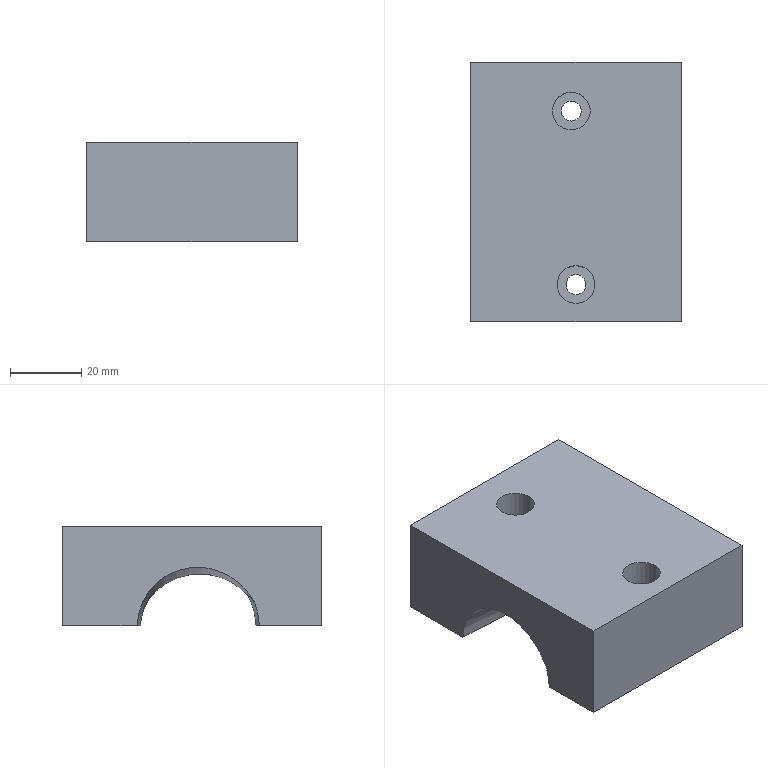NC program | NX | posted with a generic post | part box 59.014 x 72.744 x 27.972 mm
Lines 1691 to 2486 of 94199:
(FIXED_CONTOUR , TOOL : R2)
N3362 T11 M6
N3364 G54
N3366 G17 G0 G90 X17.129 Y-31.067 S9500 M3
N3368 G43 Z30. H11
N3370 Z5.2
N3372 G94 G1 Z0.147 F1000.
N3374 X17.141 Y-31.095
N3376 X17.133 Y-31.126
N3378 X17.108 Y-31.144
N3380 X17.106 Y-31.146 Z0.122 F3000.
N3382 X17.08 Y-31.172 Z-1.507
N3384 X17.056 Y-31.196 Z-2.477
N3386 X17.019 Y-31.233 Z-2.947
N3388 X16.997 Y-31.255 Z-3.192
N3390 X16.986 Y-31.266 Z-3.29
N3392 X16.964 Y-31.289 Z-3.454
N3394 X16.947 Y-31.29 Z-3.603
N3396 X16.9 Y-31.291 Z-3.934
N3398 X16.92 Y-31.272 Z-3.829
N3400 X16.962 Y-31.23 Z-3.571
N3402 X16.995 Y-31.197 Z-3.331
N3404 X17.012 Y-31.18 Z-3.182
N3406 X17.064 Y-31.127 Z-2.569
N3408 X17.076 Y-31.116 Z-2.344
N3410 X17.091 Y-31.101 Z-1.761
N3412 X17.122 Y-31.07 Z0.149
N3414 X17.127 Y-31.042 Z0.15
N3416 X17.095 Y-31.074 Z-1.856
N3418 X17.084 Y-31.085 Z-2.285
N3420 X17.067 Y-31.102 Z-2.61
N3422 X17.032 Y-31.137 Z-3.022
N3424 X17.018 Y-31.151 Z-3.175
N3426 X16.998 Y-31.171 Z-3.347
N3428 X16.969 Y-31.199 Z-3.555
N3430 X16.92 Y-31.249 Z-3.858
N3432 X16.877 Y-31.292 Z-4.088
N3434 X16.855 Y-31.293 Z-4.24
N3436 X16.92 Y-31.228 Z-3.886
N3438 X16.977 Y-31.171 Z-3.54
N3440 X17.001 Y-31.146 Z-3.361
N3442 X17.028 Y-31.119 Z-3.116
N3444 X17.043 Y-31.105 Z-2.966
N3446 X17.069 Y-31.078 Z-2.65
N3448 X17.091 Y-31.056 Z-2.23
N3450 X17.098 Y-31.049 Z-1.945
N3452 X17.132 Y-31.016 Z0.15
N3454 X17.137 Y-30.988 Z0.151
N3456 X17.102 Y-31.023 Z-2.038
N3458 X17.099 Y-31.026 Z-2.172
N3460 X17.072 Y-31.054 Z-2.691
N3462 X17.044 Y-31.082 Z-3.01
N3464 X17.019 Y-31.106 Z-3.244
N3466 X17.004 Y-31.121 Z-3.376
N3468 X16.984 Y-31.141 Z-3.524
N3470 X16.92 Y-31.206 Z-3.916
N3472 X16.851 Y-31.274 Z-4.289
N3474 X16.831 Y-31.294 Z-4.379
N3476 X16.805 Z-4.523
N3478 X16.86 Y-31.239 Z-4.276
N3480 X16.92 Y-31.179 Z-3.95
N3482 X16.993 Y-31.106 Z-3.505
N3484 X17.008 Y-31.091 Z-3.394
N3486 X17.019 Y-31.08 Z-3.295
N3488 X17.066 Y-31.033 Z-2.839
N3490 X17.074 Y-31.024 Z-2.739
N3492 X17.107 Y-30.991 Z-2.114
N3494 X17.143 Y-30.956 Z0.151
N3496 X17.149 Y-30.923 Z0.152
N3498 X17.114 Y-30.958 Z-2.091
N3500 X17.111 Y-30.961 Z-2.17
N3502 X17.077 Y-30.995 Z-2.786
N3504 X17.012 Y-31.061 Z-3.412
N3506 X17.002 Y-31.071 Z-3.486
N3508 X16.92 Y-31.153 Z-3.985
N3510 X16.869 Y-31.204 Z-4.262
N3512 X16.82 Y-31.252 Z-4.487
N3514 X16.778 Y-31.294 Z-4.665
N3516 X16.754 Y-31.295 Z-4.794
N3518 X16.82 Y-31.228 Z-4.513
N3520 X16.877 Y-31.171 Z-4.25
N3522 X16.92 Y-31.128 Z-4.017
N3524 X17.01 Y-31.038 Z-3.469
N3526 X17.019 Y-31.029 Z-3.393
N3528 X17.085 Y-30.963 Z-2.767
N3530 X17.115 Y-30.933 Z-2.207
N3532 X17.121 Y-30.927 Z-2.07
N3534 X17.155 Y-30.893 Z0.153
N3536 X17.161 Y-30.861 Z0.154
N3538 X17.127 Y-30.895 Z-2.048
N3540 X17.12 Y-30.903 Z-2.245
N3542 X17.092 Y-30.931 Z-2.755
N3544 X17.083 Y-30.94 Z-2.856
N3546 X17.018 Y-31.004 Z-3.451
N3548 X16.92 Y-31.103 Z-4.051
N3550 X16.885 Y-31.137 Z-4.238
N3552 X16.82 Y-31.203 Z-4.539
N3554 X16.752 Y-31.27 Z-4.826
N3556 X16.728 Y-31.294 Z-4.911
N3558 X16.701 Z-5.034
N3560 X16.762 Y-31.232 Z-4.815
N3562 X16.82 Y-31.174 Z-4.569
N3564 X16.895 Y-31.099 Z-4.224
N3566 X16.92 Y-31.074 Z-4.088
N3568 X16.994 Y-31. Z-3.633
N3570 X17.019 Y-30.975 Z-3.489
N3572 X17.027 Y-30.967 Z-3.435
N3574 X17.086 Y-30.908 Z-2.896
N3576 X17.1 Y-30.894 Z-2.742
N3578 X17.125 Y-30.869 Z-2.288
N3580 X17.134 Y-30.86 Z-2.023
N3582 X17.168 Y-30.826 Z0.154
N3584 X17.176 Y-30.787 Z0.155
N3586 X17.143 Y-30.82 Z-1.996
N3588 X17.13 Y-30.833 Z-2.335
N3590 X17.108 Y-30.854 Z-2.727
N3592 X17.089 Y-30.873 Z-2.94
N3594 X17.037 Y-30.925 Z-3.418
N3596 X17.019 Y-30.943 Z-3.54
N3598 X16.963 Y-31. Z-3.866
N3600 X16.92 Y-31.043 Z-4.13
N3602 X16.905 Y-31.057 Z-4.208
N3604 X16.82 Y-31.143 Z-4.602
N3606 X16.772 Y-31.19 Z-4.803
N3608 X16.669 Y-31.293 Z-5.171
N3610 X16.637 Y-31.294 Z-5.311
N3612 X16.783 Y-31.148 Z-4.792
N3614 X16.82 Y-31.111 Z-4.634
N3616 X16.92 Y-31.011 Z-4.171
N3618 X17.019 Y-30.912 Z-3.591
N3620 X17.047 Y-30.884 Z-3.402
N3622 X17.092 Y-30.839 Z-2.985
N3624 X17.117 Y-30.814 Z-2.713
N3626 X17.135 Y-30.796 Z-2.383
N3628 X17.151 Y-30.781 Z-1.969
N3630 X17.183 Y-30.748 Z0.156
N3632 X17.19 Y-30.711 Z0.157
N3634 X17.158 Y-30.743 Z-1.943
N3636 X17.14 Y-30.761 Z-2.428
N3638 X17.125 Y-30.776 Z-2.699
N3640 X17.096 Y-30.806 Z-3.026
N3642 X17.057 Y-30.845 Z-3.386
N3644 X17.019 Y-30.882 Z-3.639
N3646 X16.926 Y-30.976 Z-4.179
N3648 X16.82 Y-31.081 Z-4.665
N3650 X16.793 Y-31.109 Z-4.781
N3652 X16.62 Y-31.281 Z-5.395
N3654 X16.607 Y-31.294 Z-5.434
N3656 X16.576 Z-5.551
N3658 X16.603 Y-31.267 Z-5.468
N3660 X16.62 Y-31.249 Z-5.42
N3662 X16.643 Y-31.227 Z-5.347
N3664 X16.803 Y-31.067 Z-4.769
N3666 X16.82 Y-31.05 Z-4.698
N3668 X16.936 Y-30.934 Z-4.165
N3670 X17.019 Y-30.85 Z-3.69
N3672 X17.067 Y-30.803 Z-3.369
N3674 X17.099 Y-30.771 Z-3.071
N3676 X17.134 Y-30.736 Z-2.684
N3678 X17.146 Y-30.724 Z-2.475
N3680 X17.166 Y-30.703 Z-1.916
N3682 X17.198 Y-30.672 Z0.158
N3684 X17.206 Y-30.631
N3686 X17.175 Y-30.661 Z-1.886
N3688 X17.151 Y-30.685 Z-2.526
N3690 X17.143 Y-30.693 Z-2.669
N3692 X17.103 Y-30.734 Z-3.118
N3694 X17.077 Y-30.759 Z-3.351
N3696 X17.019 Y-30.817 Z-3.744
N3698 X16.947 Y-30.889 Z-4.15
N3700 X16.82 Y-31.016 Z-4.733
N3702 X16.66 Y-31.176 Z-5.317
N3704 X16.62 Y-31.216 Z-5.447
N3706 X16.589 Y-31.247 Z-5.531
N3708 X16.543 Y-31.293 Z-5.674
N3710 X16.508 Z-5.805
N3712 X16.575 Y-31.226 Z-5.598
N3714 X16.62 Y-31.18 Z-5.475
N3716 X16.678 Y-31.122 Z-5.284
N3718 X16.826 Y-30.975 Z-4.743
N3720 X16.92 Y-30.881 Z-4.321
N3722 X16.959 Y-30.842 Z-4.135
N3724 X17.019 Y-30.781 Z-3.798
N3726 X17.088 Y-30.712 Z-3.332
N3728 X17.106 Y-30.694 Z-3.168
N3730 X17.153 Y-30.648 Z-2.652
N3732 X17.157 Y-30.644 Z-2.579
N3734 X17.184 Y-30.617 Z-1.856
N3736 X17.214 Y-30.587 Z0.159
N3738 X17.223 Y-30.541 Z0.16
N3740 X17.192 Y-30.571 Z-1.88
N3742 X17.163 Y-30.6 Z-2.635
N3744 X17.11 Y-30.653 Z-3.22
N3746 X17.1 Y-30.663 Z-3.312
N3748 X17.019 Y-30.744 Z-3.851
N3750 X16.972 Y-30.792 Z-4.119
N3752 X16.92 Y-30.844 Z-4.363
N3754 X16.839 Y-30.925 Z-4.729
N3756 X16.82 Y-30.944 Z-4.803
N3758 X16.698 Y-31.066 Z-5.251
N3760 X16.62 Y-31.143 Z-5.504
N3762 X16.56 Y-31.204 Z-5.668
N3764 X16.47 Y-31.293 Z-5.943
N3766 X16.434 Y-31.294 Z-6.079
N3768 X16.545 Y-31.182 Z-5.736
N3770 X16.62 Y-31.107 Z-5.532
N3772 X16.716 Y-31.012 Z-5.218
N3774 X16.82 Y-30.908 Z-4.837
N3776 X16.85 Y-30.877 Z-4.716
N3778 X16.92 Y-30.808 Z-4.404
N3780 X16.983 Y-30.744 Z-4.103
N3782 X17.019 Y-30.708 Z-3.902
N3784 X17.112 Y-30.616 Z-3.293
N3786 X17.169 Y-30.558 Z-2.668
N3788 X17.174 Y-30.554 Z-2.6
N3790 X17.199 Y-30.528 Z-1.933
N3792 X17.203 Y-30.524 Z-1.758
N3794 X17.231 Y-30.496 Z0.161
N3796 X17.24 Y-30.452 Z0.162
N3798 X17.213 Y-30.48 Z-1.707
N3800 X17.207 Y-30.486 Z-1.986
N3802 X17.184 Y-30.508 Z-2.566
N3804 X17.175 Y-30.517 Z-2.702
N3806 X17.124 Y-30.568 Z-3.26
N3808 X17.118 Y-30.574 Z-3.31
N3810 X17.019 Y-30.673 Z-3.953
N3812 X16.995 Y-30.697 Z-4.088
N3814 X16.92 Y-30.773 Z-4.444
N3816 X16.862 Y-30.83 Z-4.703
N3818 X16.82 Y-30.872 Z-4.87
N3820 X16.72 Y-30.972 Z-5.234
N3822 X16.62 Y-31.072 Z-5.56
N3824 X16.531 Y-31.161 Z-5.802
N3826 X16.421 Y-31.271 Z-6.141
N3828 X16.398 Y-31.294 Z-6.197
N3830 X16.361 Z-6.315
N3832 X16.421 Y-31.234 Z-6.165
N3834 X16.516 Y-31.139 Z-5.873
N3836 X16.62 Y-31.034 Z-5.59
N3838 X16.742 Y-30.913 Z-5.193
N3840 X16.82 Y-30.835 Z-4.906
N3842 X16.875 Y-30.78 Z-4.689
N3844 X16.92 Y-30.735 Z-4.486
N3846 X17.008 Y-30.647 Z-4.071
N3848 X17.019 Y-30.635 Z-4.006
N3850 X17.122 Y-30.533 Z-3.346
N3852 X17.137 Y-30.517 Z-3.218
N3854 X17.182 Y-30.473 Z-2.737
N3856 X17.196 Y-30.459 Z-2.529
N3858 X17.214 Y-30.44 Z-2.041
N3860 X17.223 Y-30.432 Z-1.653
N3862 X17.249 Y-30.406 Z0.162
N3864 X17.258 Y-30.357 Z0.163
N3866 X17.233 Y-30.382 Z-1.595
N3868 X17.222 Y-30.393 Z-2.1
N3870 X17.207 Y-30.408 Z-2.491
N3872 X17.188 Y-30.427 Z-2.774
N3874 X17.152 Y-30.463 Z-3.173
N3876 X17.126 Y-30.489 Z-3.385
N3878 X17.02 Y-30.595 Z-4.057
N3880 X16.92 Y-30.695 Z-4.531
N3882 X16.888 Y-30.727 Z-4.674
N3884 X16.82 Y-30.795 Z-4.943
N3886 X16.755 Y-30.86 Z-5.181
N3888 X16.62 Y-30.995 Z-5.621
N3890 X16.5 Y-31.115 Z-5.948
N3892 X16.421 Y-31.194 Z-6.19
N3894 X16.322 Y-31.293 Z-6.439
N3896 X16.28 Z-6.57
N3898 X16.421 Y-31.152 Z-6.217
N3900 X16.483 Y-31.09 Z-6.028
N3902 X16.62 Y-30.952 Z-5.652
N3904 X16.636 Y-30.937 Z-5.605
N3906 X16.769 Y-30.804 Z-5.17
N3908 X16.82 Y-30.753 Z-4.983
N3910 X16.902 Y-30.671 Z-4.659
N3912 X17.029 Y-30.544 Z-4.066
N3914 X17.043 Y-30.53 Z-3.982
N3916 X17.131 Y-30.442 Z-3.426
N3918 X17.167 Y-30.406 Z-3.125
N3920 X17.195 Y-30.377 Z-2.813
N3922 X17.22 Y-30.353 Z-2.45
N3924 X17.231 Y-30.342 Z-2.162
N3926 X17.245 Y-30.328 Z-1.534
N3928 X17.268 Y-30.305 Z0.164
N3930 X17.279 Y-30.249 Z0.165
N3932 X17.257 Y-30.271 Z-1.469
N3934 X17.24 Y-30.288 Z-2.23
N3936 X17.233 Y-30.294 Z-2.406
N3938 X17.203 Y-30.324 Z-2.856
N3940 X17.183 Y-30.345 Z-3.074
N3942 X17.135 Y-30.392 Z-3.47
N3944 X17.066 Y-30.461 Z-3.911
N3946 X17.038 Y-30.489 Z-4.076
N3948 X16.917 Y-30.61 Z-4.642
N3950 X16.82 Y-30.708 Z-5.025
N3952 X16.784 Y-30.743 Z-5.157
N3954 X16.72 Y-30.807 Z-5.371
N3956 X16.651 Y-30.876 Z-5.594
N3958 X16.62 Y-30.907 Z-5.686
N3960 X16.464 Y-31.063 Z-6.113
N3962 X16.421 Y-31.107 Z-6.247
N3964 X16.314 Y-31.213 Z-6.513
N3966 X16.234 Y-31.293 Z-6.704
N3968 X16.189 Z-6.83
N3970 X16.221 Y-31.26 Z-6.76
N3972 X16.36 Y-31.122 Z-6.429
N3974 X16.421 Y-31.061 Z-6.276
N3976 X16.446 Y-31.036 Z-6.2
N3978 X16.62 Y-30.861 Z-5.72
N3980 X16.666 Y-30.815 Z-5.582
N3982 X16.799 Y-30.682 Z-5.144
N3984 X16.82 Y-30.662 Z-5.068
N3986 X16.932 Y-30.549 Z-4.625
N3988 X17.047 Y-30.434 Z-4.086
N3990 X17.089 Y-30.392 Z-3.839
N3992 X17.14 Y-30.342 Z-3.515
N3994 X17.199 Y-30.282 Z-3.022
N3996 X17.211 Y-30.271 Z-2.898
N3998 X17.247 Y-30.235 Z-2.362
N4000 X17.249 Y-30.233 Z-2.297
N4002 X17.27 Y-30.212 Z-1.346
N4004 X17.29 Y-30.192 Z0.166
N4006 X17.301 Y-30.134 Z0.167
N4008 X17.28 Y-30.155 Z-1.441
N4010 X17.259 Y-30.176 Z-2.352
N4012 X17.216 Y-30.219 Z-2.969
N4014 X17.145 Y-30.29 Z-3.561
N4016 X17.113 Y-30.322 Z-3.765
N4018 X17.057 Y-30.378 Z-4.096
N4020 X16.948 Y-30.487 Z-4.608
N4022 X16.815 Y-30.62 Z-5.131
N4024 X16.682 Y-30.753 Z-5.571
N4026 X16.62 Y-30.815 Z-5.755
N4028 X16.421 Y-31.014 Z-6.306
N4030 X16.221 Y-31.214 Z-6.787
N4032 X16.189 Y-31.246 Z-6.854
N4034 X16.142 Y-31.293 Z-6.958
N4036 X16.094 Z-7.089
N4038 X16.17 Y-31.217 Z-6.921
N4040 X16.221 Y-31.166 Z-6.815
N4042 X16.421 Y-30.966 Z-6.337
N4044 X16.454 Y-30.933 Z-6.248
N4046 X16.62 Y-30.767 Z-5.791
N4048 X16.698 Y-30.689 Z-5.559
N4050 X16.831 Y-30.556 Z-5.116
N4052 X16.92 Y-30.468 Z-4.77
N4054 X16.964 Y-30.423 Z-4.59
N4056 X17.066 Y-30.321 Z-4.107
N4058 X17.15 Y-30.237 Z-3.607
N4060 X17.227 Y-30.16 Z-2.98
N4062 X17.233 Y-30.154 Z-2.912
N4064 X17.268 Y-30.119 Z-2.389
N4066 X17.274 Y-30.113 Z-2.227
N4068 X17.29 Y-30.097 Z-1.507
N4070 X17.312 Y-30.075 Z0.169
N4072 X17.324 Y-30.015 Z0.17
N4074 X17.301 Y-30.038 Z-1.574
N4076 X17.288 Y-30.051 Z-2.151
N4078 X17.278 Y-30.061 Z-2.426
N4080 X17.249 Y-30.09 Z-2.854
N4082 X17.235 Y-30.104 Z-3.016
N4084 X17.155 Y-30.184 Z-3.652
N4086 X17.076 Y-30.263 Z-4.117
N4088 X16.98 Y-30.359 Z-4.572
N4090 X16.92 Y-30.419 Z-4.817
N4092 X16.847 Y-30.492 Z-5.101
N4094 X16.82 Y-30.519 Z-5.195
N4096 X16.714 Y-30.625 Z-5.547
N4098 X16.62 Y-30.719 Z-5.827
N4100 X16.502 Y-30.837 Z-6.152
N4102 X16.421 Y-30.918 Z-6.367
N4104 X16.339 Y-31. Z-6.559
N4106 X16.221 Y-31.118 Z-6.843
N4108 X16.15 Y-31.189 Z-6.99
N4110 X16.046 Y-31.293 Z-7.223
N4112 X16.022 Y-31.294 Z-7.288
N4114 X15.994 Z-7.357
N4116 X16.022 Y-31.266 Z-7.302
N4118 X16.13 Y-31.158 Z-7.062
N4120 X16.221 Y-31.067 Z-6.873
N4122 X16.288 Y-31. Z-6.711
N4124 X16.421 Y-30.867 Z-6.4
N4126 X16.553 Y-30.735 Z-6.05
N4128 X16.62 Y-30.668 Z-5.865
N4130 X16.731 Y-30.557 Z-5.534
N4132 X16.82 Y-30.468 Z-5.239
N4134 X16.864 Y-30.424 Z-5.084
N4136 X16.92 Y-30.368 Z-4.867
N4138 X16.997 Y-30.291 Z-4.553
N4140 X17.086 Y-30.202 Z-4.128
N4142 X17.161 Y-30.127 Z-3.695
N4144 X17.184 Y-30.104 Z-3.534
N4146 X17.243 Y-30.045 Z-3.053
N4148 X17.266 Y-30.022 Z-2.792
N4150 X17.288 Y-30. Z-2.465
N4152 X17.302 Y-29.986 Z-2.07
N4154 X17.312 Y-29.976 Z-1.644
N4156 X17.336 Y-29.952 Z0.171
N4158 X17.348 Y-29.89 Z0.172
N4160 X17.323 Y-29.915 Z-1.714
N4162 X17.317 Y-29.921 Z-1.99
N4164 X17.299 Y-29.939 Z-2.504
N4166 X17.283 Y-29.955 Z-2.731
N4168 X17.252 Y-29.986 Z-3.091
N4170 X17.207 Y-30.031 Z-3.455
N4172 X17.166 Y-30.071 Z-3.737
N4174 X17.105 Y-30.133 Z-4.096
N4176 X17.089 Y-30.149 Z-4.176
N4178 X17.014 Y-30.224 Z-4.534
N4180 X16.92 Y-30.318 Z-4.916
N4182 X16.881 Y-30.357 Z-5.068
N4184 X16.82 Y-30.418 Z-5.282
N4186 X16.748 Y-30.49 Z-5.521
N4188 X16.62 Y-30.617 Z-5.903
N4190 X16.421 Y-30.817 Z-6.432
N4192 X16.221 Y-31.016 Z-6.902
N4194 X16.094 Y-31.144 Z-7.167
N4196 X16.022 Y-31.216 Z-7.328
N4198 X15.943 Y-31.294 Z-7.481
N4200 X15.895 Z-7.6
N4202 X16.022 Y-31.168 Z-7.353
N4204 X16.09 Y-31.1 Z-7.201
N4206 X16.221 Y-30.968 Z-6.93
N4208 X16.421 Y-30.769 Z-6.463
N4210 X16.62 Y-30.569 Z-5.938
N4212 X16.764 Y-30.426 Z-5.509
N4214 X16.82 Y-30.37 Z-5.323
N4216 X16.897 Y-30.293 Z-5.053
N4218 X17.028 Y-30.162 Z-4.524
N4220 X17.091 Y-30.098 Z-4.221
N4222 X17.122 Y-30.068 Z-4.066
N4224 X17.171 Y-30.018 Z-3.778
N4226 X17.229 Y-29.961 Z-3.379
N4228 X17.26 Y-29.929 Z-3.127
N4230 X17.299 Y-29.89 Z-2.672
N4232 X17.308 Y-29.881 Z-2.541
N4234 X17.331 Y-29.859 Z-1.913
N4236 X17.333 Y-29.856 Z-1.781
N4238 X17.359 Y-29.83 Z0.173
N4240 X17.371 Y-29.771 Z0.174
N4242 X17.344 Y-29.797 Z-1.845
N4244 X17.318 Y-29.824 Z-2.578
N4246 X17.268 Y-29.873 Z-3.162
N4248 X17.251 Y-29.891 Z-3.304
N4250 X17.176 Y-29.965 Z-3.818
N4252 X17.139 Y-30.003 Z-4.035
N4254 X17.094 Y-30.048 Z-4.267
N4256 X17.041 Y-30.1 Z-4.518
N4258 X16.913 Y-30.229 Z-5.038
N4260 X16.82 Y-30.322 Z-5.363
N4262 X16.78 Y-30.362 Z-5.497
N4264 X16.62 Y-30.521 Z-5.971
N4266 X16.541 Y-30.6 Z-6.176
N4268 X16.421 Y-30.721 Z-6.494
N4270 X16.301 Y-30.841 Z-6.776
N4272 X16.221 Y-30.92 Z-6.957
N4274 X16.07 Y-31.071 Z-7.269
N4276 X16.022 Y-31.12 Z-7.378
N4278 X15.902 Y-31.239 Z-7.612
N4280 X15.848 Y-31.294 Z-7.714
N4282 X15.798 Y-31.293 Z-7.826
N4284 X15.952 Y-31.14 Z-7.54
N4286 X16.022 Y-31.07 Z-7.403
N4288 X16.05 Y-31.042 Z-7.34
N4290 X16.221 Y-30.871 Z-6.985
N4292 X16.35 Y-30.742 Z-6.692
N4294 X16.421 Y-30.671 Z-6.526
N4296 X16.492 Y-30.6 Z-6.338
N4298 X16.62 Y-30.472 Z-6.006
N4300 X16.796 Y-30.296 Z-5.484
N4302 X16.82 Y-30.272 Z-5.405
N4304 X16.929 Y-30.163 Z-5.022
N4306 X17.055 Y-30.037 Z-4.512
N4308 X17.096 Y-29.996 Z-4.314
N4310 X17.157 Y-29.935 Z-4.004
N4312 X17.182 Y-29.91 Z-3.859
N4314 X17.276 Y-29.815 Z-3.199
N4316 X17.329 Y-29.763 Z-2.603
N4318 X17.356 Y-29.736 Z-1.882
N4320 X17.383 Y-29.709 Z0.175
N4322 X17.395 Y-29.645 Z0.176
N4324 X17.367 Y-29.673 Z-1.921
N4326 X17.348 Y-29.692 Z-2.454
N4328 X17.34 Y-29.7 Z-2.621
N4330 X17.29 Y-29.75 Z-3.189
N4332 X17.283 Y-29.757 Z-3.248
N4334 X17.187 Y-29.853 Z-3.903
N4336 X17.175 Y-29.865 Z-3.971
N4338 X17.099 Y-29.941 Z-4.363
N4340 X17.069 Y-29.971 Z-4.506
N4342 X16.946 Y-30.094 Z-5.005
N4344 X16.813 Y-30.227 Z-5.471
N4346 X16.62 Y-30.42 Z-6.043
N4348 X16.421 Y-30.619 Z-6.559
N4350 X16.221 Y-30.819 Z-7.015
N4352 X16.003 Y-31.037 Z-7.466
N4354 X15.822 Y-31.218 Z-7.808
N4356 X15.792 Y-31.249 Z-7.86
N4358 X15.747 Y-31.293 Z-7.941
N4360 X15.694 Y-31.292 Z-8.062
N4362 X15.77 Y-31.216 Z-7.923
N4364 X15.822 Y-31.164 Z-7.834
N4366 X16.022 Y-30.965 Z-7.457
N4368 X16.221 Y-30.765 Z-7.045
N4370 X16.421 Y-30.566 Z-6.592
N4372 X16.456 Y-30.531 Z-6.506
N4374 X16.62 Y-30.366 Z-6.081
N4376 X16.831 Y-30.155 Z-5.456
N4378 X16.92 Y-30.067 Z-5.149
N4380 X16.964 Y-30.022 Z-4.988
N4382 X17.084 Y-29.903 Z-4.499
N4384 X17.102 Y-29.885 Z-4.414
N4386 X17.196 Y-29.791 Z-3.931
N4388 X17.289 Y-29.698 Z-3.302
N4390 X17.306 Y-29.681 Z-3.164
N4392 X17.352 Y-29.635 Z-2.64
N4394 X17.365 Y-29.621 Z-2.364
N4396 X17.38 Y-29.606 Z-1.962
N4398 X17.408 Y-29.579 Z0.178
N4400 X17.421 Y-29.511 Z0.179
N4402 X17.393 Y-29.539 Z-2.004
N4404 X17.383 Y-29.548 Z-2.272
N4406 X17.364 Y-29.568 Z-2.659
N4408 X17.322 Y-29.61 Z-3.139
N4410 X17.295 Y-29.636 Z-3.357
N4412 X17.221 Y-29.71 Z-3.856
N4414 X17.197 Y-29.735 Z-4.
N4416 X17.099 Y-29.832 Z-4.492
N4418 X16.983 Y-29.949 Z-4.97
N4420 X16.92 Y-30.012 Z-5.197
N4422 X16.85 Y-30.082 Z-5.441
N4424 X16.82 Y-30.111 Z-5.535
N4426 X16.73 Y-30.201 Z-5.794
N4428 X16.62 Y-30.311 Z-6.12
N4430 X16.511 Y-30.421 Z-6.403
N4432 X16.421 Y-30.51 Z-6.626
N4434 X16.221 Y-30.71 Z-7.077
N4436 X16.112 Y-30.819 Z-7.304
N4438 X16.022 Y-30.909 Z-7.485
N4440 X15.822 Y-31.109 Z-7.861
N4442 X15.748 Y-31.184 Z-7.988
N4444 X15.638 Y-31.293 Z-8.188
N4446 X15.586 Y-31.294 Z-8.296
N4448 X15.623 Y-31.257 Z-8.238
N4450 X15.727 Y-31.153 Z-8.048
N4452 X15.822 Y-31.057 Z-7.886
N4454 X16.022 Y-30.858 Z-7.512
N4456 X16.163 Y-30.717 Z-7.227
N4458 X16.221 Y-30.658 Z-7.106
N4460 X16.421 Y-30.459 Z-6.657
N4462 X16.562 Y-30.318 Z-6.306
N4464 X16.62 Y-30.259 Z-6.156
N4466 X16.679 Y-30.201 Z-5.983
N4468 X16.82 Y-30.06 Z-5.575
N4470 X16.867 Y-30.013 Z-5.426
N4472 X16.92 Y-29.96 Z-5.242
N4474 X17. Y-29.88 Z-4.954
N4476 X17.117 Y-29.763 Z-4.469
N4478 X17.2 Y-29.68 Z-4.047
N4480 X17.245 Y-29.635 Z-3.786
N4482 X17.301 Y-29.579 Z-3.409
N4484 X17.337 Y-29.543 Z-3.115
N4486 X17.375 Y-29.505 Z-2.677
N4488 X17.399 Y-29.48 Z-2.186
N4490 X17.405 Y-29.475 Z-2.043
N4492 X17.433 Y-29.447 Z0.18
N4494 X17.445 Y-29.383 Z0.181
N4496 X17.416 Y-29.412 Z-2.1
N4498 X17.386 Y-29.442 Z-2.695
N4500 X17.352 Y-29.476 Z-3.092
N4502 X17.307 Y-29.522 Z-3.461
N4504 X17.269 Y-29.559 Z-3.715
N4506 X17.204 Y-29.624 Z-4.095
N4508 X17.137 Y-29.691 Z-4.433
N4510 X17.108 Y-29.72 Z-4.561
N4512 X17.017 Y-29.811 Z-4.937
N4514 X16.884 Y-29.944 Z-5.411
N4516 X16.82 Y-30.008 Z-5.616
N4518 X16.614 Y-30.215 Z-6.21
N4520 X16.421 Y-30.407 Z-6.688
N4522 X16.215 Y-30.613 Z-7.149
N4524 X16.022 Y-30.806 Z-7.538
N4526 X15.822 Y-31.006 Z-7.911
N4528 X15.706 Y-31.122 Z-8.108
N4530 X15.623 Y-31.205 Z-8.26
N4532 X15.535 Y-31.293 Z-8.4
N4534 X15.483 Z-8.504
N4536 X15.623 Y-31.153 Z-8.283
N4538 X15.685 Y-31.091 Z-8.169
N4540 X15.822 Y-30.954 Z-7.936
N4542 X16.022 Y-30.754 Z-7.565
N4544 X16.221 Y-30.555 Z-7.164
N4546 X16.267 Y-30.51 Z-7.065
N4548 X16.421 Y-30.355 Z-6.72
N4550 X16.62 Y-30.156 Z-6.227
N4552 X16.665 Y-30.111 Z-6.102
N4554 X16.82 Y-29.956 Z-5.656
N4556 X16.901 Y-29.875 Z-5.397
N4558 X17.034 Y-29.742 Z-4.921
N4560 X17.11 Y-29.666 Z-4.609
N4562 X17.158 Y-29.619 Z-4.397
N4564 X17.208 Y-29.569 Z-4.143
N4566 X17.293 Y-29.483 Z-3.644
N4568 X17.312 Y-29.464 Z-3.513
N4570 X17.367 Y-29.409 Z-3.068
N4572 X17.4 Y-29.376 Z-2.683
N4574 X17.418 Y-29.358 Z-2.364
N4576 X17.429 Y-29.347 Z-2.072
N4578 X17.458 Y-29.319 Z0.182
N4580 X17.47 Y-29.254 Z0.184
N4582 X17.441 Y-29.283 Z-2.113
N4584 X17.427 Y-29.297 Z-2.435
N4586 X17.417 Y-29.307 Z-2.621
N4588 X17.404 Y-29.321 Z-2.8
N4590 X17.378 Y-29.347 Z-3.085
N4592 X17.317 Y-29.407 Z-3.573
N4594 X17.211 Y-29.513 Z-4.192
N4596 X17.178 Y-29.546 Z-4.36
N4598 X17.112 Y-29.612 Z-4.656
N4600 X17.052 Y-29.673 Z-4.904
N4602 X16.919 Y-29.806 Z-5.382
N4604 X16.82 Y-29.905 Z-5.696
N4606 X16.717 Y-30.007 Z-5.993
N4608 X16.62 Y-30.104 Z-6.261
N4610 X16.421 Y-30.303 Z-6.752
N4612 X16.319 Y-30.406 Z-6.981
N4614 X16.221 Y-30.503 Z-7.192
N4616 X16.022 Y-30.702 Z-7.592
N4618 X15.822 Y-30.902 Z-7.961
N4620 X15.664 Y-31.06 Z-8.23
N4622 X15.623 Y-31.101 Z-8.305
N4624 X15.431 Y-31.293 Z-8.608
N4626 X15.377 Z-8.712
N4628 X15.423 Y-31.247 Z-8.643
N4630 X15.623 Y-31.048 Z-8.328
N4632 X15.642 Y-31.028 Z-8.293
N4634 X15.822 Y-30.848 Z-7.986
N4636 X16.022 Y-30.649 Z-7.619
N4638 X16.221 Y-30.449 Z-7.221
N4640 X16.372 Y-30.298 Z-6.893
N4642 X16.421 Y-30.25 Z-6.785
N4644 X16.62 Y-30.05 Z-6.296
N4646 X16.771 Y-29.899 Z-5.879
N4648 X16.82 Y-29.851 Z-5.738
N4650 X16.937 Y-29.734 Z-5.367
N4652 X17.019 Y-29.651 Z-5.072
N4654 X17.07 Y-29.601 Z-4.888
N4656 X17.114 Y-29.557 Z-4.705
N4658 X17.199 Y-29.471 Z-4.322
N4660 X17.215 Y-29.455 Z-4.242
N4662 X17.319 Y-29.352 Z-3.643
N4664 X17.335 Y-29.335 Z-3.535
N4666 X17.389 Y-29.282 Z-3.108
N4668 X17.402 Y-29.269 Z-2.979
N4670 X17.411 Y-29.259 Z-2.871
N4672 X17.43 Y-29.24 Z-2.62
N4674 X17.446 Y-29.224 Z-2.315
N4676 X17.453 Y-29.217 Z-2.127
N4678 X17.483 Y-29.188 Z0.185
N4680 X17.496 Y-29.118 Z0.186
N4682 X17.467 Y-29.148 Z-2.142
N4684 X17.462 Y-29.153 Z-2.269
N4686 X17.443 Y-29.171 Z-2.624
N4688 X17.42 Y-29.194 Z-2.936
N4690 X17.4 Y-29.215 Z-3.132
N4692 X17.354 Y-29.26 Z-3.498
N4694 X17.319 Y-29.296 Z-3.725
N4696 X17.221 Y-29.393 Z-4.284
N4698 X17.116 Y-29.498 Z-4.756
N4700 X17.088 Y-29.526 Z-4.87
N4702 X17.019 Y-29.595 Z-5.124
N4704 X16.955 Y-29.659 Z-5.352
N4706 X16.82 Y-29.794 Z-5.782
N4708 X16.62 Y-29.994 Z-6.333
N4710 X16.421 Y-30.193 Z-6.819
N4712 X16.221 Y-30.393 Z-7.252
N4714 X16.014 Y-30.6 Z-7.662
N4716 X15.822 Y-30.792 Z-8.013
N4718 X15.623 Y-30.991 Z-8.352
N4720 X15.423 Y-31.191 Z-8.667
N4722 X15.383 Y-31.231 Z-8.726
N4724 X15.322 Y-31.293 Z-8.82
N4726 X15.263 Z-8.932
N4728 X15.359 Y-31.197 Z-8.785
N4730 X15.423 Y-31.133 Z-8.692
N4732 X15.623 Y-30.933 Z-8.378
N4734 X15.822 Y-30.734 Z-8.041
N4736 X16.022 Y-30.534 Z-7.677
N4738 X16.221 Y-30.335 Z-7.283
N4740 X16.421 Y-30.135 Z-6.852
N4742 X16.487 Y-30.069 Z-6.697
N4744 X16.62 Y-29.936 Z-6.371
N4746 X16.754 Y-29.802 Z-6.
N4748 X16.82 Y-29.736 Z-5.824
N4750 X16.975 Y-29.581 Z-5.336
N4752 X17.108 Y-29.448 Z-4.852
N4754 X17.241 Y-29.316 Z-4.258
N4756 X17.319 Y-29.237 Z-3.81
N4758 X17.374 Y-29.183 Z-3.46
N4760 X17.411 Y-29.145 Z-3.157
N4762 X17.434 Y-29.123 Z-2.936
N4764 X17.457 Y-29.099 Z-2.628
N4766 X17.48 Y-29.076 Z-2.158
N4768 X17.51 Y-29.046 Z0.187
N4770 X17.525 Y-28.97 Z0.189
N4772 X17.495 Y-29. Z-2.173
N4774 X17.469 Y-29.026 Z-2.668
N4776 X17.448 Y-29.047 Z-2.936
N4778 X17.418 Y-29.076 Z-3.226
N4780 X17.394 Y-29.1 Z-3.419
N4782 X17.319 Y-29.176 Z-3.9
N4784 X17.261 Y-29.233 Z-4.23
N4786 X17.128 Y-29.366 Z-4.831
N4788 X16.995 Y-29.499 Z-5.319
N4790 X16.82 Y-29.675 Z-5.869
N4792 X16.693 Y-29.802 Z-6.211
N4794 X16.62 Y-29.874 Z-6.411
N4796 X16.548 Y-29.946 Z-6.587
N4798 X16.421 Y-30.074 Z-6.888
N4800 X16.221 Y-30.273 Z-7.317
N4802 X16.022 Y-30.473 Z-7.708
N4804 X15.822 Y-30.672 Z-8.071
N4806 X15.623 Y-30.872 Z-8.406
N4808 X15.423 Y-31.071 Z-8.718
N4810 X15.334 Y-31.16 Z-8.848
N4812 X15.224 Y-31.271 Z-9.017
N4814 X15.201 Y-31.294 Z-9.048
N4816 X15.138 Z-9.159
N4818 X15.224 Y-31.208 Z-9.041
N4820 X15.309 Y-31.123 Z-8.912
N4822 X15.432 Y-31. Z-8.731
N4824 X15.623 Y-30.809 Z-8.434
N4826 X15.831 Y-30.6 Z-8.085
N4828 X16.022 Y-30.41 Z-7.74
N4830 X16.221 Y-30.21 Z-7.351
N4832 X16.421 Y-30.011 Z-6.924
N4834 X16.62 Y-29.811 Z-6.453
N4836 X16.82 Y-29.612 Z-5.915
N4838 X17.019 Y-29.412 Z-5.29
N4840 X17.149 Y-29.283 Z-4.809
N4842 X17.209 Y-29.223 Z-4.531
N4844 X17.282 Y-29.15 Z-4.202
N4846 X17.319 Y-29.113 Z-3.992
N4848 X17.418 Y-29.013 Z-3.351
N4850 X17.463 Y-28.969 Z-2.932
N4852 X17.486 Y-28.946 Z-2.63
N4854 X17.509 Y-28.923 Z-2.173
N4856 X17.54 Y-28.892 Z0.19
N4858 X17.554 Y-28.817 Z0.192
N4860 X17.527 Y-28.844 Z-1.89
N4862 X17.523 Y-28.848 Z-2.173
N4864 X17.5 Y-28.871 Z-2.625
N4866 X17.477 Y-28.895 Z-2.924
N4868 X17.43 Y-28.941 Z-3.369
N4870 X17.418 Y-28.953 Z-3.45
N4872 X17.319 Y-29.053 Z-4.08
N4874 X17.302 Y-29.069 Z-4.175
N4876 X17.169 Y-29.202 Z-4.788
N4878 X17.036 Y-29.335 Z-5.284
N4880 X17.019 Y-29.352 Z-5.341
N4882 X16.969 Y-29.402 Z-5.494
N4884 X16.82 Y-29.551 Z-5.959
N4886 X16.671 Y-29.7 Z-6.359
N4888 X16.62 Y-29.751 Z-6.491
N4890 X16.421 Y-29.95 Z-6.959
N4892 X16.221 Y-30.15 Z-7.383
N4894 X16.022 Y-30.349 Z-7.77
N4896 X15.822 Y-30.549 Z-8.129
N4898 X15.623 Y-30.748 Z-8.46
N4900 X15.423 Y-30.948 Z-8.77
N4902 X15.284 Y-31.087 Z-8.973
N4904 X15.224 Y-31.147 Z-9.065
N4906 X15.077 Y-31.294 Z-9.266
N4908 X15.019 Z-9.368
N4910 X15.224 Y-31.089 Z-9.088
N4912 X15.26 Y-31.053 Z-9.032
N4914 X15.423 Y-30.89 Z-8.795
N4916 X15.623 Y-30.69 Z-8.486
N4918 X15.822 Y-30.491 Z-8.157
N4920 X16.022 Y-30.291 Z-7.8
N4922 X16.221 Y-30.092 Z-7.414
N4924 X16.421 Y-29.892 Z-6.993
N4926 X16.511 Y-29.802 Z-6.78
N4928 X16.62 Y-29.693 Z-6.528
N4930 X16.729 Y-29.584 Z-6.245
N4932 X16.82 Y-29.493 Z-6.002
N4934 X16.91 Y-29.402 Z-5.719
N4936 X17.019 Y-29.294 Z-5.389
N4938 X17.056 Y-29.257 Z-5.267
N4940 X17.189 Y-29.124 Z-4.767
N4942 X17.322 Y-28.991 Z-4.148
N4944 X17.418 Y-28.895 Z-3.541
N4946 X17.444 Y-28.869 Z-3.365